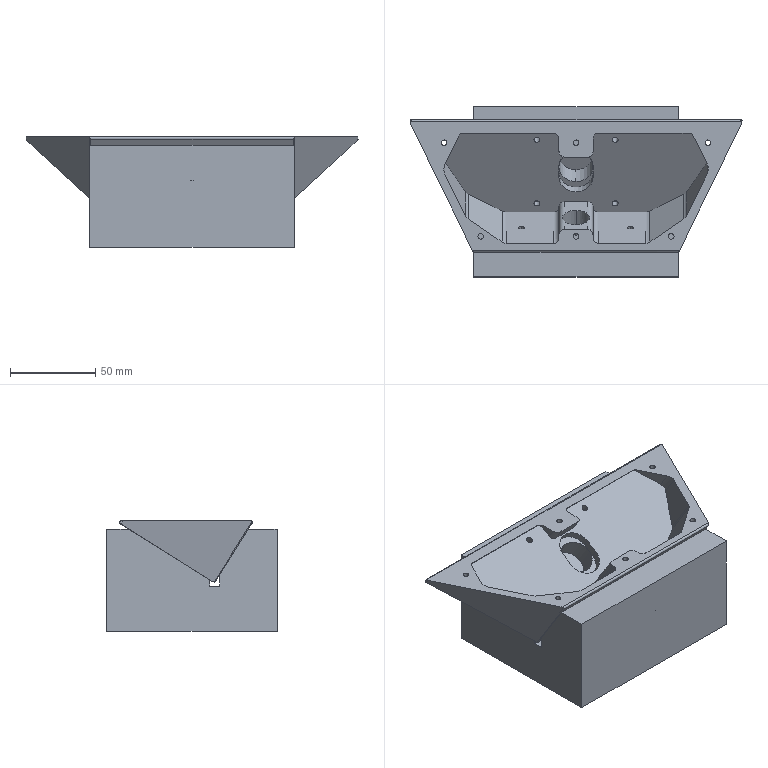NC program | Mastercam | posted with a generic post | part box 195.124 x 100 x 65 mm
Whole program:
%
O0000()
(MATERIAL - ALUMINUM MM - 2024)
( T3 | 6 SPD | H3 )
N100 G21
N110 G0 G17 G40 G49 G80 G90
N120 T3 M6
N130 G0 G90 G54 X0. Y29.731 A0. S3000 M3
N140 G43 H3 Z30.
N150 G98 G81 Z-1.65 R1. F300.
N160 Y-25.269
N170 G80
N180 M5
N190 G91 G0 G28 Z0.
N200 G28 X0. Y0. A0.
N210 M30
%